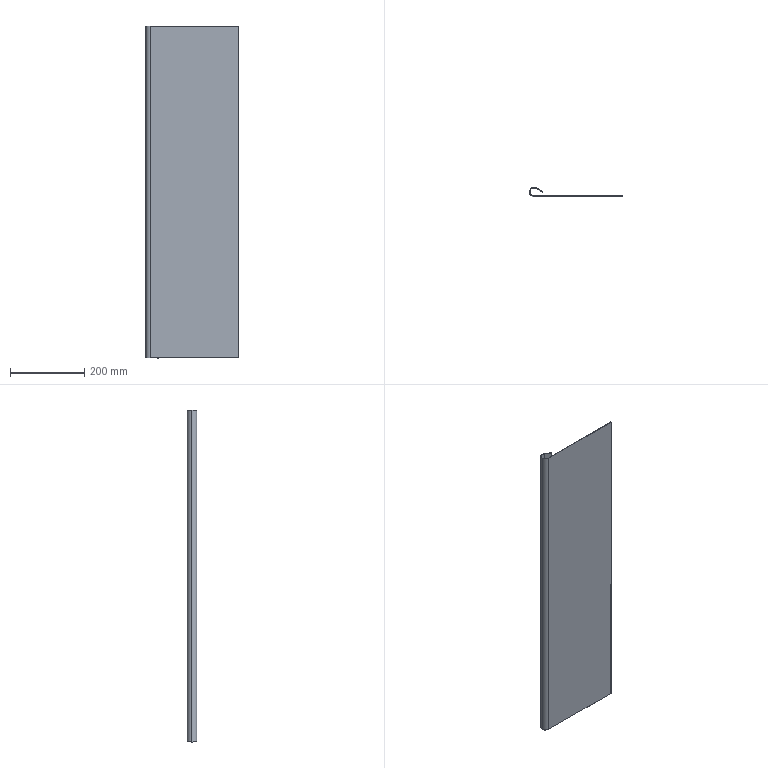Part | STEP file | 750078465 | 1 solid | 12 faces | box 250 x 25 x 892.6 mm | volume 322531 mm3 | plane 8 | cylinder 4 | commonest cylinder face diameters 22.6 x2 25 x2
STEP:
#1=CARTESIAN_POINT('',(1.2,12.5,446.3));
#2=VERTEX_POINT('',#1);
#3=CARTESIAN_POINT('',(18.15,22.286,446.3));
#4=VERTEX_POINT('',#3);
#5=CARTESIAN_POINT('',(12.5,12.5,446.3));
#6=DIRECTION('',(0.,0.,-1.));
#7=DIRECTION('',(-1.,0.,0.));
#8=AXIS2_PLACEMENT_3D('',#5,#6,#7);
#9=CIRCLE('',#8,11.3);
#10=EDGE_CURVE('',#2,#4,#9,.T.);
#11=ORIENTED_EDGE('',*,*,#10,.F.);
#12=CARTESIAN_POINT('',(1.2,12.5,-446.3));
#13=VERTEX_POINT('',#12);
#14=CARTESIAN_POINT('',(1.2,12.5,446.3));
#15=DIRECTION('',(0.,0.,-1.));
#16=VECTOR('',#15,1000.);
#17=LINE('',#14,#16);
#18=EDGE_CURVE('',#2,#13,#17,.T.);
#19=ORIENTED_EDGE('',*,*,#18,.T.);
#20=CARTESIAN_POINT('',(18.15,22.286,-446.3));
#21=VERTEX_POINT('',#20);
#22=CARTESIAN_POINT('',(12.5,12.5,-446.3));
#23=DIRECTION('',(0.,0.,1.));
#24=DIRECTION('',(-1.,0.,0.));
#25=AXIS2_PLACEMENT_3D('',#22,#23,#24);
#26=CIRCLE('',#25,11.3);
#27=EDGE_CURVE('',#21,#13,#26,.T.);
#28=ORIENTED_EDGE('',*,*,#27,.F.);
#29=CARTESIAN_POINT('',(18.15,22.286,446.3));
#30=DIRECTION('',(0.,0.,-1.));
#31=VECTOR('',#30,1000.);
#32=LINE('',#29,#31);
#33=EDGE_CURVE('',#4,#21,#32,.T.);
#34=ORIENTED_EDGE('',*,*,#33,.F.);
#35=EDGE_LOOP('',(#11,#19,#28,#34));
#36=FACE_OUTER_BOUND('',#35,.T.);
#37=CARTESIAN_POINT('',(12.5,12.5,446.3));
#38=DIRECTION('',(0.,0.,-1.));
#39=DIRECTION('',(-1.,0.,0.));
#40=AXIS2_PLACEMENT_3D('',#37,#38,#39);
#41=CYLINDRICAL_SURFACE('',#40,11.3);
#42=ADVANCED_FACE('',(#36),#41,.F.);
#43=CARTESIAN_POINT('',(0.,12.5,446.3));
#44=VERTEX_POINT('',#43);
#45=CARTESIAN_POINT('',(12.5,0.,446.3));
#46=VERTEX_POINT('',#45);
#47=CARTESIAN_POINT('',(12.5,12.5,446.3));
#48=DIRECTION('',(0.,0.,1.));
#49=DIRECTION('',(-1.,0.,0.));
#50=AXIS2_PLACEMENT_3D('',#47,#48,#49);
#51=CIRCLE('',#50,12.5);
#52=EDGE_CURVE('',#44,#46,#51,.T.);
#53=ORIENTED_EDGE('',*,*,#52,.F.);
#54=CARTESIAN_POINT('',(0.,12.5,-446.3));
#55=VERTEX_POINT('',#54);
#56=CARTESIAN_POINT('',(0.,12.5,446.3));
#57=DIRECTION('',(0.,0.,-1.));
#58=VECTOR('',#57,1000.);
#59=LINE('',#56,#58);
#60=EDGE_CURVE('',#44,#55,#59,.T.);
#61=ORIENTED_EDGE('',*,*,#60,.T.);
#62=CARTESIAN_POINT('',(12.5,0.,-446.3));
#63=VERTEX_POINT('',#62);
#64=CARTESIAN_POINT('',(12.5,12.5,-446.3));
#65=DIRECTION('',(0.,0.,1.));
#66=DIRECTION('',(-1.,0.,0.));
#67=AXIS2_PLACEMENT_3D('',#64,#65,#66);
#68=CIRCLE('',#67,12.5);
#69=EDGE_CURVE('',#55,#63,#68,.T.);
#70=ORIENTED_EDGE('',*,*,#69,.T.);
#71=CARTESIAN_POINT('',(12.5,0.,446.3));
#72=DIRECTION('',(0.,0.,1.));
#73=VECTOR('',#72,1000.);
#74=LINE('',#71,#73);
#75=EDGE_CURVE('',#63,#46,#74,.T.);
#76=ORIENTED_EDGE('',*,*,#75,.T.);
#77=EDGE_LOOP('',(#53,#61,#70,#76));
#78=FACE_OUTER_BOUND('',#77,.T.);
#79=CARTESIAN_POINT('',(12.5,12.5,446.3));
#80=DIRECTION('',(0.,0.,-1.));
#81=DIRECTION('',(-1.,0.,0.));
#82=AXIS2_PLACEMENT_3D('',#79,#80,#81);
#83=CYLINDRICAL_SURFACE('',#82,12.5);
#84=ADVANCED_FACE('',(#78),#83,.T.);
#85=CARTESIAN_POINT('',(12.5,1.2,446.3));
#86=VERTEX_POINT('',#85);
#87=CARTESIAN_POINT('',(250.,1.2,446.3));
#88=VERTEX_POINT('',#87);
#89=CARTESIAN_POINT('',(12.5,1.2,446.3));
#90=DIRECTION('',(1.,0.,0.));
#91=VECTOR('',#90,1000.);
#92=LINE('',#89,#91);
#93=EDGE_CURVE('',#86,#88,#92,.T.);
#94=ORIENTED_EDGE('',*,*,#93,.T.);
#95=CARTESIAN_POINT('',(250.,1.2,-446.3));
#96=VERTEX_POINT('',#95);
#97=CARTESIAN_POINT('',(250.,1.2,446.3));
#98=DIRECTION('',(0.,0.,-1.));
#99=VECTOR('',#98,1000.);
#100=LINE('',#97,#99);
#101=EDGE_CURVE('',#88,#96,#100,.T.);
#102=ORIENTED_EDGE('',*,*,#101,.T.);
#103=CARTESIAN_POINT('',(12.5,1.2,-446.3));
#104=VERTEX_POINT('',#103);
#105=CARTESIAN_POINT('',(12.5,1.2,-446.3));
#106=DIRECTION('',(-1.,0.,0.));
#107=VECTOR('',#106,1000.);
#108=LINE('',#105,#107);
#109=EDGE_CURVE('',#96,#104,#108,.T.);
#110=ORIENTED_EDGE('',*,*,#109,.T.);
#111=CARTESIAN_POINT('',(12.5,1.2,446.3));
#112=DIRECTION('',(0.,0.,1.));
#113=VECTOR('',#112,1000.);
#114=LINE('',#111,#113);
#115=EDGE_CURVE('',#104,#86,#114,.T.);
#116=ORIENTED_EDGE('',*,*,#115,.T.);
#117=EDGE_LOOP('',(#94,#102,#110,#116));
#118=FACE_OUTER_BOUND('',#117,.T.);
#119=CARTESIAN_POINT('',(12.5,1.2,446.3));
#120=DIRECTION('',(0.,1.,0.));
#121=DIRECTION('',(0.,0.,1.));
#122=AXIS2_PLACEMENT_3D('',#119,#120,#121);
#123=PLANE('',#122);
#124=ADVANCED_FACE('',(#118),#123,.T.);
#125=CARTESIAN_POINT('',(250.,0.,-446.3));
#126=VERTEX_POINT('',#125);
#127=CARTESIAN_POINT('',(250.,0.,-446.3));
#128=DIRECTION('',(0.,1.,0.));
#129=VECTOR('',#128,1000.);
#130=LINE('',#127,#129);
#131=EDGE_CURVE('',#126,#96,#130,.T.);
#132=ORIENTED_EDGE('',*,*,#131,.T.);
#133=ORIENTED_EDGE('',*,*,#101,.F.);
#134=CARTESIAN_POINT('',(250.,0.,446.3));
#135=VERTEX_POINT('',#134);
#136=CARTESIAN_POINT('',(250.,0.,446.3));
#137=DIRECTION('',(0.,-1.,0.));
#138=VECTOR('',#137,1000.);
#139=LINE('',#136,#138);
#140=EDGE_CURVE('',#88,#135,#139,.T.);
#141=ORIENTED_EDGE('',*,*,#140,.T.);
#142=CARTESIAN_POINT('',(250.,0.,446.3));
#143=DIRECTION('',(0.,0.,-1.));
#144=VECTOR('',#143,1000.);
#145=LINE('',#142,#144);
#146=EDGE_CURVE('',#135,#126,#145,.T.);
#147=ORIENTED_EDGE('',*,*,#146,.T.);
#148=EDGE_LOOP('',(#132,#133,#141,#147));
#149=FACE_OUTER_BOUND('',#148,.T.);
#150=CARTESIAN_POINT('',(250.,0.,446.3));
#151=DIRECTION('',(1.,0.,0.));
#152=DIRECTION('',(0.,0.,-1.));
#153=AXIS2_PLACEMENT_3D('',#150,#151,#152);
#154=PLANE('',#153);
#155=ADVANCED_FACE('',(#149),#154,.T.);
#156=CARTESIAN_POINT('',(12.5,0.,446.3));
#157=DIRECTION('',(1.,0.,0.));
#158=VECTOR('',#157,1000.);
#159=LINE('',#156,#158);
#160=EDGE_CURVE('',#46,#135,#159,.T.);
#161=ORIENTED_EDGE('',*,*,#160,.T.);
#162=ORIENTED_EDGE('',*,*,#140,.F.);
#163=ORIENTED_EDGE('',*,*,#93,.F.);
#164=CARTESIAN_POINT('',(12.5,12.5,446.3));
#165=DIRECTION('',(0.,0.,-1.));
#166=DIRECTION('',(-1.,0.,0.));
#167=AXIS2_PLACEMENT_3D('',#164,#165,#166);
#168=CIRCLE('',#167,11.3);
#169=EDGE_CURVE('',#86,#2,#168,.T.);
#170=ORIENTED_EDGE('',*,*,#169,.T.);
#171=ORIENTED_EDGE('',*,*,#10,.T.);
#172=CARTESIAN_POINT('',(35.471,12.286,446.3));
#173=VERTEX_POINT('',#172);
#174=CARTESIAN_POINT('',(18.15,22.286,446.3));
#175=DIRECTION('',(0.866,-0.5,0.));
#176=VECTOR('',#175,1000.);
#177=LINE('',#174,#176);
#178=EDGE_CURVE('',#4,#173,#177,.T.);
#179=ORIENTED_EDGE('',*,*,#178,.T.);
#180=CARTESIAN_POINT('',(36.071,13.325,446.3));
#181=VERTEX_POINT('',#180);
#182=CARTESIAN_POINT('',(36.071,13.325,446.3));
#183=DIRECTION('',(0.5,0.866,0.));
#184=VECTOR('',#183,1000.);
#185=LINE('',#182,#184);
#186=EDGE_CURVE('',#173,#181,#185,.T.);
#187=ORIENTED_EDGE('',*,*,#186,.T.);
#188=CARTESIAN_POINT('',(18.75,23.325,446.3));
#189=VERTEX_POINT('',#188);
#190=CARTESIAN_POINT('',(36.071,13.325,446.3));
#191=DIRECTION('',(-0.866,0.5,0.));
#192=VECTOR('',#191,1000.);
#193=LINE('',#190,#192);
#194=EDGE_CURVE('',#181,#189,#193,.T.);
#195=ORIENTED_EDGE('',*,*,#194,.T.);
#196=CARTESIAN_POINT('',(12.5,12.5,446.3));
#197=DIRECTION('',(0.,0.,1.));
#198=DIRECTION('',(-1.,0.,0.));
#199=AXIS2_PLACEMENT_3D('',#196,#197,#198);
#200=CIRCLE('',#199,12.5);
#201=EDGE_CURVE('',#189,#44,#200,.T.);
#202=ORIENTED_EDGE('',*,*,#201,.T.);
#203=ORIENTED_EDGE('',*,*,#52,.T.);
#204=EDGE_LOOP('',(#161,#162,#163,#170,#171,#179,#187,#195,#202,#203));
#205=FACE_OUTER_BOUND('',#204,.T.);
#206=CARTESIAN_POINT('',(12.5,0.,446.3));
#207=DIRECTION('',(0.,0.,1.));
#208=DIRECTION('',(1.,0.,0.));
#209=AXIS2_PLACEMENT_3D('',#206,#207,#208);
#210=PLANE('',#209);
#211=ADVANCED_FACE('',(#205),#210,.T.);
#212=ORIENTED_EDGE('',*,*,#18,.F.);
#213=ORIENTED_EDGE('',*,*,#169,.F.);
#214=ORIENTED_EDGE('',*,*,#115,.F.);
#215=CARTESIAN_POINT('',(12.5,12.5,-446.3));
#216=DIRECTION('',(0.,0.,1.));
#217=DIRECTION('',(-1.,0.,0.));
#218=AXIS2_PLACEMENT_3D('',#215,#216,#217);
#219=CIRCLE('',#218,11.3);
#220=EDGE_CURVE('',#13,#104,#219,.T.);
#221=ORIENTED_EDGE('',*,*,#220,.F.);
#222=EDGE_LOOP('',(#212,#213,#214,#221));
#223=FACE_OUTER_BOUND('',#222,.T.);
#224=CARTESIAN_POINT('',(12.5,12.5,446.3));
#225=DIRECTION('',(0.,0.,-1.));
#226=DIRECTION('',(-1.,0.,0.));
#227=AXIS2_PLACEMENT_3D('',#224,#225,#226);
#228=CYLINDRICAL_SURFACE('',#227,11.3);
#229=ADVANCED_FACE('',(#223),#228,.F.);
#230=ORIENTED_EDGE('',*,*,#27,.T.);
#231=ORIENTED_EDGE('',*,*,#220,.T.);
#232=ORIENTED_EDGE('',*,*,#109,.F.);
#233=ORIENTED_EDGE('',*,*,#131,.F.);
#234=CARTESIAN_POINT('',(36.071,0.,-446.3));
#235=DIRECTION('',(1.,0.,0.));
#236=VECTOR('',#235,1000.);
#237=LINE('',#234,#236);
#238=EDGE_CURVE('',#63,#126,#237,.T.);
#239=ORIENTED_EDGE('',*,*,#238,.F.);
#240=ORIENTED_EDGE('',*,*,#69,.F.);
#241=CARTESIAN_POINT('',(18.75,23.325,-446.3));
#242=VERTEX_POINT('',#241);
#243=CARTESIAN_POINT('',(12.5,12.5,-446.3));
#244=DIRECTION('',(0.,0.,1.));
#245=DIRECTION('',(-1.,0.,0.));
#246=AXIS2_PLACEMENT_3D('',#243,#244,#245);
#247=CIRCLE('',#246,12.5);
#248=EDGE_CURVE('',#242,#55,#247,.T.);
#249=ORIENTED_EDGE('',*,*,#248,.F.);
#250=CARTESIAN_POINT('',(36.071,13.325,-446.3));
#251=VERTEX_POINT('',#250);
#252=CARTESIAN_POINT('',(36.071,13.325,-446.3));
#253=DIRECTION('',(-0.866,0.5,0.));
#254=VECTOR('',#253,1000.);
#255=LINE('',#252,#254);
#256=EDGE_CURVE('',#251,#242,#255,.T.);
#257=ORIENTED_EDGE('',*,*,#256,.F.);
#258=CARTESIAN_POINT('',(35.471,12.286,-446.3));
#259=VERTEX_POINT('',#258);
#260=CARTESIAN_POINT('',(36.071,13.325,-446.3));
#261=DIRECTION('',(-0.5,-0.866,0.));
#262=VECTOR('',#261,1000.);
#263=LINE('',#260,#262);
#264=EDGE_CURVE('',#251,#259,#263,.T.);
#265=ORIENTED_EDGE('',*,*,#264,.T.);
#266=CARTESIAN_POINT('',(18.15,22.286,-446.3));
#267=DIRECTION('',(0.866,-0.5,0.));
#268=VECTOR('',#267,1000.);
#269=LINE('',#266,#268);
#270=EDGE_CURVE('',#21,#259,#269,.T.);
#271=ORIENTED_EDGE('',*,*,#270,.F.);
#272=EDGE_LOOP('',(#230,#231,#232,#233,#239,#240,#249,#257,#265,#271));
#273=FACE_OUTER_BOUND('',#272,.T.);
#274=CARTESIAN_POINT('',(36.071,13.325,-446.3));
#275=DIRECTION('',(0.,0.,1.));
#276=DIRECTION('',(1.,0.,0.));
#277=AXIS2_PLACEMENT_3D('',#274,#275,#276);
#278=PLANE('',#277);
#279=ADVANCED_FACE('',(#273),#278,.F.);
#280=ORIENTED_EDGE('',*,*,#146,.F.);
#281=ORIENTED_EDGE('',*,*,#160,.F.);
#282=ORIENTED_EDGE('',*,*,#75,.F.);
#283=ORIENTED_EDGE('',*,*,#238,.T.);
#284=EDGE_LOOP('',(#280,#281,#282,#283));
#285=FACE_OUTER_BOUND('',#284,.T.);
#286=CARTESIAN_POINT('',(12.5,0.,446.3));
#287=DIRECTION('',(0.,1.,0.));
#288=DIRECTION('',(0.,0.,1.));
#289=AXIS2_PLACEMENT_3D('',#286,#287,#288);
#290=PLANE('',#289);
#291=ADVANCED_FACE('',(#285),#290,.F.);
#292=ORIENTED_EDGE('',*,*,#60,.F.);
#293=ORIENTED_EDGE('',*,*,#201,.F.);
#294=CARTESIAN_POINT('',(18.75,23.325,446.3));
#295=DIRECTION('',(0.,0.,-1.));
#296=VECTOR('',#295,1000.);
#297=LINE('',#294,#296);
#298=EDGE_CURVE('',#189,#242,#297,.T.);
#299=ORIENTED_EDGE('',*,*,#298,.T.);
#300=ORIENTED_EDGE('',*,*,#248,.T.);
#301=EDGE_LOOP('',(#292,#293,#299,#300));
#302=FACE_OUTER_BOUND('',#301,.T.);
#303=CARTESIAN_POINT('',(12.5,12.5,446.3));
#304=DIRECTION('',(0.,0.,-1.));
#305=DIRECTION('',(-1.,0.,0.));
#306=AXIS2_PLACEMENT_3D('',#303,#304,#305);
#307=CYLINDRICAL_SURFACE('',#306,12.5);
#308=ADVANCED_FACE('',(#302),#307,.T.);
#309=ORIENTED_EDGE('',*,*,#298,.F.);
#310=ORIENTED_EDGE('',*,*,#194,.F.);
#311=CARTESIAN_POINT('',(36.071,13.325,446.3));
#312=DIRECTION('',(0.,0.,1.));
#313=VECTOR('',#312,1000.);
#314=LINE('',#311,#313);
#315=EDGE_CURVE('',#251,#181,#314,.T.);
#316=ORIENTED_EDGE('',*,*,#315,.F.);
#317=ORIENTED_EDGE('',*,*,#256,.T.);
#318=EDGE_LOOP('',(#309,#310,#316,#317));
#319=FACE_OUTER_BOUND('',#318,.T.);
#320=CARTESIAN_POINT('',(36.071,13.325,446.3));
#321=DIRECTION('',(-0.5,-0.866,0.));
#322=DIRECTION('',(0.866,-0.5,0.));
#323=AXIS2_PLACEMENT_3D('',#320,#321,#322);
#324=PLANE('',#323);
#325=ADVANCED_FACE('',(#319),#324,.F.);
#326=ORIENTED_EDGE('',*,*,#178,.F.);
#327=ORIENTED_EDGE('',*,*,#33,.T.);
#328=ORIENTED_EDGE('',*,*,#270,.T.);
#329=CARTESIAN_POINT('',(35.471,12.286,446.3));
#330=DIRECTION('',(0.,0.,1.));
#331=VECTOR('',#330,1000.);
#332=LINE('',#329,#331);
#333=EDGE_CURVE('',#259,#173,#332,.T.);
#334=ORIENTED_EDGE('',*,*,#333,.T.);
#335=EDGE_LOOP('',(#326,#327,#328,#334));
#336=FACE_OUTER_BOUND('',#335,.T.);
#337=CARTESIAN_POINT('',(35.471,12.286,446.3));
#338=DIRECTION('',(-0.5,-0.866,0.));
#339=DIRECTION('',(0.866,-0.5,0.));
#340=AXIS2_PLACEMENT_3D('',#337,#338,#339);
#341=PLANE('',#340);
#342=ADVANCED_FACE('',(#336),#341,.T.);
#343=ORIENTED_EDGE('',*,*,#186,.F.);
#344=ORIENTED_EDGE('',*,*,#333,.F.);
#345=ORIENTED_EDGE('',*,*,#264,.F.);
#346=ORIENTED_EDGE('',*,*,#315,.T.);
#347=EDGE_LOOP('',(#343,#344,#345,#346));
#348=FACE_OUTER_BOUND('',#347,.T.);
#349=CARTESIAN_POINT('',(36.071,13.325,446.3));
#350=DIRECTION('',(-0.866,0.5,0.));
#351=DIRECTION('',(-0.5,-0.866,0.));
#352=AXIS2_PLACEMENT_3D('',#349,#350,#351);
#353=PLANE('',#352);
#354=ADVANCED_FACE('',(#348),#353,.F.);
#355=CLOSED_SHELL('',(#42,#84,#124,#155,#211,#229,#279,#291,#308,#325,#342,#354));
#356=MANIFOLD_SOLID_BREP('',#355);
#357=CARTESIAN_POINT('',(0.,0.,0.));
#358=DIRECTION('',(0.,0.,1.));
#359=DIRECTION('',(1.,0.,0.));
#360=AXIS2_PLACEMENT_3D('',#357,#358,#359);
#361=(LENGTH_UNIT()NAMED_UNIT(*)SI_UNIT(.MILLI.,.METRE.));
#362=UNCERTAINTY_MEASURE_WITH_UNIT(LENGTH_MEASURE(0.00001),#361,'','');
#363=(NAMED_UNIT(*)PLANE_ANGLE_UNIT()SI_UNIT($,.RADIAN.));
#364=(NAMED_UNIT(*)SI_UNIT($,.STERADIAN.)SOLID_ANGLE_UNIT());
#365=(GEOMETRIC_REPRESENTATION_CONTEXT(3)GLOBAL_UNCERTAINTY_ASSIGNED_CONTEXT((#362))GLOBAL_UNIT_ASSIGNED_CONTEXT((#361,#363,#364))REPRESENTATION_CONTEXT('',''));
#366=ADVANCED_BREP_SHAPE_REPRESENTATION('',(#356,#360),#365);